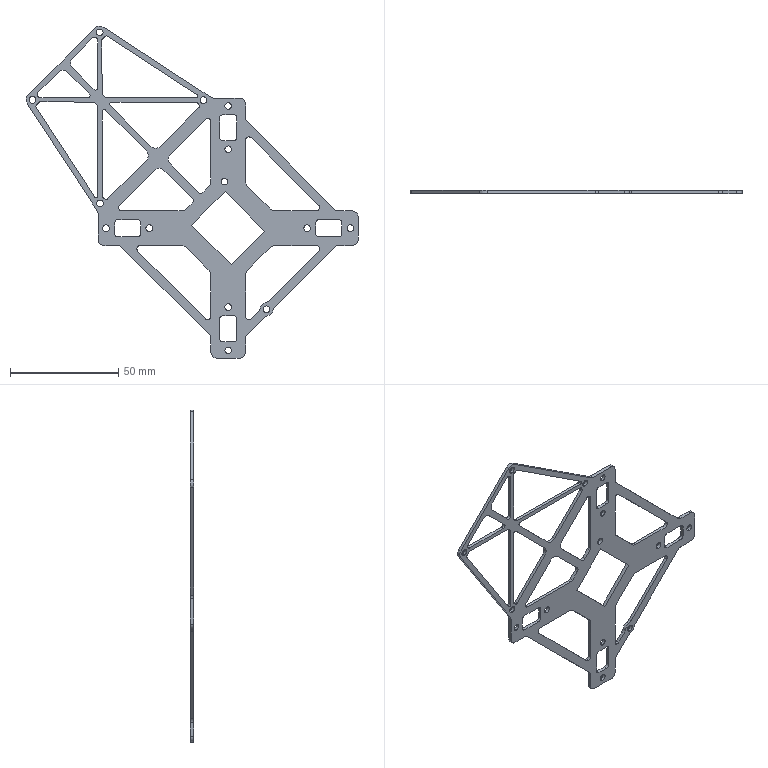Part | SolidWorks | features Fillet 4, Extrusion 1, ICE 1 | 1 solid | 205 faces | box 153.518 x 1.5 x 153.518 mm | volume 7437 mm3 | cylinder 127 | plane 78 | commonest cylinder face diameters 3 x31 6 x29 3.1 x28 2 x25 5 x14